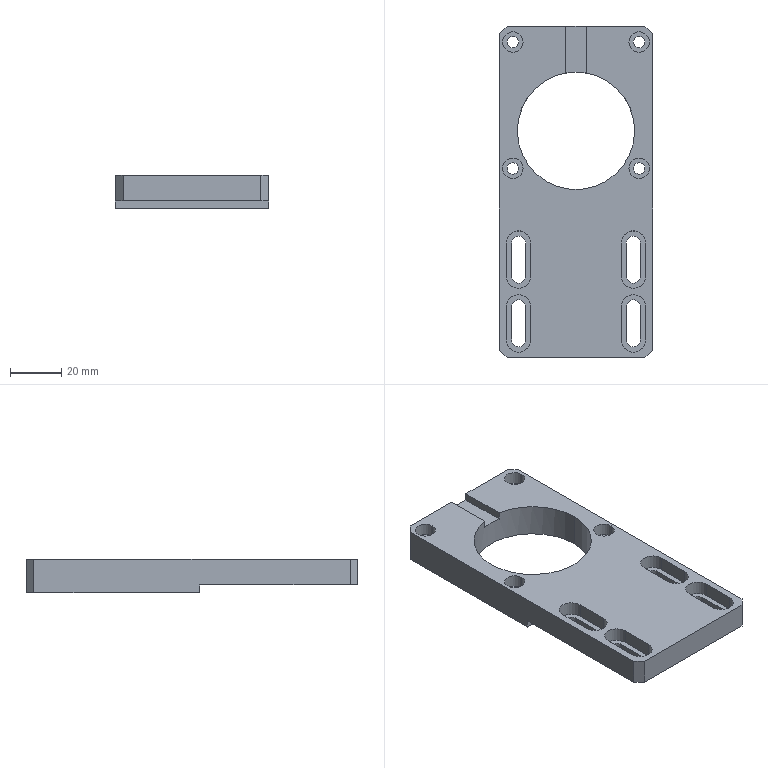Part | STEP file | 10000020558swp000-1 | 1 solid | 73 faces | box 60 x 130 x 13 mm | volume 60488 mm3 | plane 39 | cylinder 34 | commonest cylinder face diameters 4.5 x8 5.5 x8 8 x8 9.5 x8 46 x2